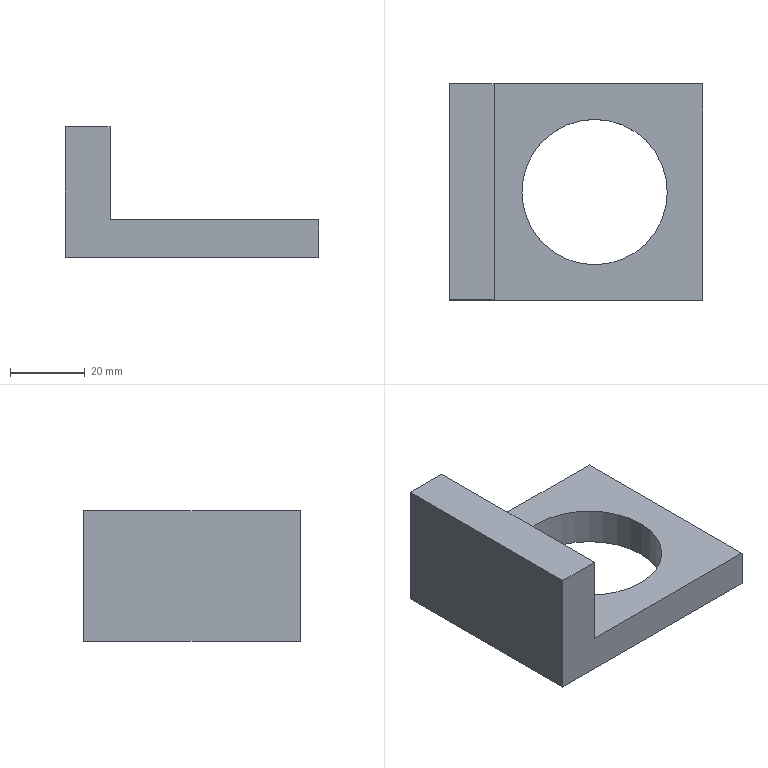Part | SolidWorks | features ICE 3, Extrusion 1 | 1 solid | 10 faces | box 68 x 58 x 35 mm | volume 44894 mm3 | plane 8 | cylinder 2 | commonest cylinder face diameters 39 x2
STEP:
#1=CARTESIAN_POINT('',(19.5,29.,0.));
#2=VERTEX_POINT('',#1);
#3=CARTESIAN_POINT('',(58.5,29.,0.));
#4=VERTEX_POINT('',#3);
#5=CARTESIAN_POINT('',(39.,29.,0.));
#6=DIRECTION('',(0.,0.,1.));
#7=DIRECTION('',(-1.,0.,0.));
#8=AXIS2_PLACEMENT_3D('',#5,#6,#7);
#9=CIRCLE('',#8,19.5);
#10=EDGE_CURVE('',#2,#4,#9,.T.);
#11=ORIENTED_EDGE('',*,*,#10,.F.);
#12=CARTESIAN_POINT('',(19.5,29.,10.));
#13=VERTEX_POINT('',#12);
#14=CARTESIAN_POINT('',(19.5,29.,-0.001));
#15=DIRECTION('',(0.,0.,1.));
#16=VECTOR('',#15,1000.);
#17=LINE('',#14,#16);
#18=EDGE_CURVE('',#2,#13,#17,.T.);
#19=ORIENTED_EDGE('',*,*,#18,.T.);
#20=CARTESIAN_POINT('',(58.5,29.,10.));
#21=VERTEX_POINT('',#20);
#22=CARTESIAN_POINT('',(39.,29.,10.));
#23=DIRECTION('',(0.,0.,1.));
#24=DIRECTION('',(1.,0.,0.));
#25=AXIS2_PLACEMENT_3D('',#22,#23,#24);
#26=CIRCLE('',#25,19.5);
#27=EDGE_CURVE('',#13,#21,#26,.T.);
#28=ORIENTED_EDGE('',*,*,#27,.T.);
#29=CARTESIAN_POINT('',(58.5,29.,-0.001));
#30=DIRECTION('',(0.,0.,1.));
#31=VECTOR('',#30,1000.);
#32=LINE('',#29,#31);
#33=EDGE_CURVE('',#4,#21,#32,.T.);
#34=ORIENTED_EDGE('',*,*,#33,.F.);
#35=EDGE_LOOP('',(#11,#19,#28,#34));
#36=FACE_OUTER_BOUND('',#35,.T.);
#37=CARTESIAN_POINT('',(39.,29.,-0.001));
#38=DIRECTION('',(0.,0.,1.));
#39=DIRECTION('',(1.,0.,0.));
#40=AXIS2_PLACEMENT_3D('',#37,#38,#39);
#41=CYLINDRICAL_SURFACE('',#40,19.5);
#42=ADVANCED_FACE('',(#36),#41,.F.);
#43=CARTESIAN_POINT('',(39.,29.,10.));
#44=DIRECTION('',(0.,0.,1.));
#45=DIRECTION('',(1.,0.,0.));
#46=AXIS2_PLACEMENT_3D('',#43,#44,#45);
#47=CIRCLE('',#46,19.5);
#48=EDGE_CURVE('',#21,#13,#47,.T.);
#49=ORIENTED_EDGE('',*,*,#48,.F.);
#50=ORIENTED_EDGE('',*,*,#27,.F.);
#51=EDGE_LOOP('',(#49,#50));
#52=FACE_BOUND('',#51,.T.);
#53=CARTESIAN_POINT('',(12.,0.,10.));
#54=VERTEX_POINT('',#53);
#55=CARTESIAN_POINT('',(12.,58.,10.));
#56=VERTEX_POINT('',#55);
#57=CARTESIAN_POINT('',(12.,58.,10.));
#58=DIRECTION('',(0.,1.,0.));
#59=VECTOR('',#58,1000.);
#60=LINE('',#57,#59);
#61=EDGE_CURVE('',#54,#56,#60,.T.);
#62=ORIENTED_EDGE('',*,*,#61,.F.);
#63=CARTESIAN_POINT('',(68.,0.,10.));
#64=VERTEX_POINT('',#63);
#65=CARTESIAN_POINT('',(68.,0.,10.));
#66=DIRECTION('',(1.,0.,0.));
#67=VECTOR('',#66,1000.);
#68=LINE('',#65,#67);
#69=EDGE_CURVE('',#54,#64,#68,.T.);
#70=ORIENTED_EDGE('',*,*,#69,.T.);
#71=CARTESIAN_POINT('',(68.,58.,10.));
#72=VERTEX_POINT('',#71);
#73=CARTESIAN_POINT('',(68.,58.,10.));
#74=DIRECTION('',(0.,1.,0.));
#75=VECTOR('',#74,1000.);
#76=LINE('',#73,#75);
#77=EDGE_CURVE('',#64,#72,#76,.T.);
#78=ORIENTED_EDGE('',*,*,#77,.T.);
#79=CARTESIAN_POINT('',(0.,58.,10.));
#80=DIRECTION('',(-1.,0.,0.));
#81=VECTOR('',#80,1000.);
#82=LINE('',#79,#81);
#83=EDGE_CURVE('',#72,#56,#82,.T.);
#84=ORIENTED_EDGE('',*,*,#83,.T.);
#85=EDGE_LOOP('',(#62,#70,#78,#84));
#86=FACE_OUTER_BOUND('',#85,.T.);
#87=CARTESIAN_POINT('',(0.,0.,10.));
#88=DIRECTION('',(0.,0.,-1.));
#89=DIRECTION('',(-1.,0.,0.));
#90=AXIS2_PLACEMENT_3D('',#87,#88,#89);
#91=PLANE('',#90);
#92=ADVANCED_FACE('',(#52,#86),#91,.F.);
#93=CARTESIAN_POINT('',(0.,0.,0.));
#94=VERTEX_POINT('',#93);
#95=CARTESIAN_POINT('',(68.,0.,0.));
#96=VERTEX_POINT('',#95);
#97=CARTESIAN_POINT('',(68.,0.,0.));
#98=DIRECTION('',(1.,0.,0.));
#99=VECTOR('',#98,1000.);
#100=LINE('',#97,#99);
#101=EDGE_CURVE('',#94,#96,#100,.T.);
#102=ORIENTED_EDGE('',*,*,#101,.T.);
#103=CARTESIAN_POINT('',(68.,0.,10.));
#104=DIRECTION('',(0.,0.,-1.));
#105=VECTOR('',#104,1000.);
#106=LINE('',#103,#105);
#107=EDGE_CURVE('',#64,#96,#106,.T.);
#108=ORIENTED_EDGE('',*,*,#107,.F.);
#109=ORIENTED_EDGE('',*,*,#69,.F.);
#110=CARTESIAN_POINT('',(12.,0.,35.));
#111=VERTEX_POINT('',#110);
#112=CARTESIAN_POINT('',(12.,0.,35.));
#113=DIRECTION('',(0.,0.,-1.));
#114=VECTOR('',#113,1000.);
#115=LINE('',#112,#114);
#116=EDGE_CURVE('',#111,#54,#115,.T.);
#117=ORIENTED_EDGE('',*,*,#116,.F.);
#118=CARTESIAN_POINT('',(0.,0.,35.));
#119=VERTEX_POINT('',#118);
#120=CARTESIAN_POINT('',(0.,0.,35.));
#121=DIRECTION('',(1.,0.,0.));
#122=VECTOR('',#121,1000.);
#123=LINE('',#120,#122);
#124=EDGE_CURVE('',#119,#111,#123,.T.);
#125=ORIENTED_EDGE('',*,*,#124,.F.);
#126=CARTESIAN_POINT('',(0.,0.,10.));
#127=DIRECTION('',(0.,0.,-1.));
#128=VECTOR('',#127,1000.);
#129=LINE('',#126,#128);
#130=EDGE_CURVE('',#119,#94,#129,.T.);
#131=ORIENTED_EDGE('',*,*,#130,.T.);
#132=EDGE_LOOP('',(#102,#108,#109,#117,#125,#131));
#133=FACE_OUTER_BOUND('',#132,.T.);
#134=CARTESIAN_POINT('',(68.,0.,10.));
#135=DIRECTION('',(0.,1.,0.));
#136=DIRECTION('',(-1.,0.,0.));
#137=AXIS2_PLACEMENT_3D('',#134,#135,#136);
#138=PLANE('',#137);
#139=ADVANCED_FACE('',(#133),#138,.F.);
#140=CARTESIAN_POINT('',(68.,58.,0.));
#141=VERTEX_POINT('',#140);
#142=CARTESIAN_POINT('',(68.,58.,0.));
#143=DIRECTION('',(0.,1.,0.));
#144=VECTOR('',#143,1000.);
#145=LINE('',#142,#144);
#146=EDGE_CURVE('',#96,#141,#145,.T.);
#147=ORIENTED_EDGE('',*,*,#146,.T.);
#148=CARTESIAN_POINT('',(68.,58.,10.));
#149=DIRECTION('',(0.,0.,-1.));
#150=VECTOR('',#149,1000.);
#151=LINE('',#148,#150);
#152=EDGE_CURVE('',#72,#141,#151,.T.);
#153=ORIENTED_EDGE('',*,*,#152,.F.);
#154=ORIENTED_EDGE('',*,*,#77,.F.);
#155=ORIENTED_EDGE('',*,*,#107,.T.);
#156=EDGE_LOOP('',(#147,#153,#154,#155));
#157=FACE_OUTER_BOUND('',#156,.T.);
#158=CARTESIAN_POINT('',(68.,58.,10.));
#159=DIRECTION('',(-1.,0.,0.));
#160=DIRECTION('',(0.,0.,1.));
#161=AXIS2_PLACEMENT_3D('',#158,#159,#160);
#162=PLANE('',#161);
#163=ADVANCED_FACE('',(#157),#162,.F.);
#164=CARTESIAN_POINT('',(0.,58.,0.));
#165=VERTEX_POINT('',#164);
#166=CARTESIAN_POINT('',(0.,58.,0.));
#167=DIRECTION('',(-1.,0.,0.));
#168=VECTOR('',#167,1000.);
#169=LINE('',#166,#168);
#170=EDGE_CURVE('',#141,#165,#169,.T.);
#171=ORIENTED_EDGE('',*,*,#170,.T.);
#172=CARTESIAN_POINT('',(0.,58.,35.));
#173=VERTEX_POINT('',#172);
#174=CARTESIAN_POINT('',(0.,58.,10.));
#175=DIRECTION('',(0.,0.,-1.));
#176=VECTOR('',#175,1000.);
#177=LINE('',#174,#176);
#178=EDGE_CURVE('',#173,#165,#177,.T.);
#179=ORIENTED_EDGE('',*,*,#178,.F.);
#180=CARTESIAN_POINT('',(12.,58.,35.));
#181=VERTEX_POINT('',#180);
#182=CARTESIAN_POINT('',(0.,58.,35.));
#183=DIRECTION('',(-1.,0.,0.));
#184=VECTOR('',#183,1000.);
#185=LINE('',#182,#184);
#186=EDGE_CURVE('',#181,#173,#185,.T.);
#187=ORIENTED_EDGE('',*,*,#186,.F.);
#188=CARTESIAN_POINT('',(12.,58.,35.));
#189=DIRECTION('',(0.,0.,-1.));
#190=VECTOR('',#189,1000.);
#191=LINE('',#188,#190);
#192=EDGE_CURVE('',#181,#56,#191,.T.);
#193=ORIENTED_EDGE('',*,*,#192,.T.);
#194=ORIENTED_EDGE('',*,*,#83,.F.);
#195=ORIENTED_EDGE('',*,*,#152,.T.);
#196=EDGE_LOOP('',(#171,#179,#187,#193,#194,#195));
#197=FACE_OUTER_BOUND('',#196,.T.);
#198=CARTESIAN_POINT('',(0.,58.,10.));
#199=DIRECTION('',(0.,-1.,0.));
#200=DIRECTION('',(1.,0.,0.));
#201=AXIS2_PLACEMENT_3D('',#198,#199,#200);
#202=PLANE('',#201);
#203=ADVANCED_FACE('',(#197),#202,.F.);
#204=CARTESIAN_POINT('',(0.,0.,0.));
#205=DIRECTION('',(0.,-1.,0.));
#206=VECTOR('',#205,1000.);
#207=LINE('',#204,#206);
#208=EDGE_CURVE('',#165,#94,#207,.T.);
#209=ORIENTED_EDGE('',*,*,#208,.T.);
#210=ORIENTED_EDGE('',*,*,#130,.F.);
#211=CARTESIAN_POINT('',(0.,58.,35.));
#212=DIRECTION('',(0.,-1.,0.));
#213=VECTOR('',#212,1000.);
#214=LINE('',#211,#213);
#215=EDGE_CURVE('',#173,#119,#214,.T.);
#216=ORIENTED_EDGE('',*,*,#215,.F.);
#217=ORIENTED_EDGE('',*,*,#178,.T.);
#218=EDGE_LOOP('',(#209,#210,#216,#217));
#219=FACE_OUTER_BOUND('',#218,.T.);
#220=CARTESIAN_POINT('',(0.,0.,10.));
#221=DIRECTION('',(1.,0.,0.));
#222=DIRECTION('',(0.,0.,-1.));
#223=AXIS2_PLACEMENT_3D('',#220,#221,#222);
#224=PLANE('',#223);
#225=ADVANCED_FACE('',(#219),#224,.F.);
#226=CARTESIAN_POINT('',(39.,29.,0.));
#227=DIRECTION('',(0.,0.,1.));
#228=DIRECTION('',(-1.,0.,0.));
#229=AXIS2_PLACEMENT_3D('',#226,#227,#228);
#230=CIRCLE('',#229,19.5);
#231=EDGE_CURVE('',#4,#2,#230,.T.);
#232=ORIENTED_EDGE('',*,*,#231,.T.);
#233=ORIENTED_EDGE('',*,*,#10,.T.);
#234=EDGE_LOOP('',(#232,#233));
#235=FACE_BOUND('',#234,.T.);
#236=ORIENTED_EDGE('',*,*,#101,.F.);
#237=ORIENTED_EDGE('',*,*,#208,.F.);
#238=ORIENTED_EDGE('',*,*,#170,.F.);
#239=ORIENTED_EDGE('',*,*,#146,.F.);
#240=EDGE_LOOP('',(#236,#237,#238,#239));
#241=FACE_OUTER_BOUND('',#240,.T.);
#242=CARTESIAN_POINT('',(0.,0.,0.));
#243=DIRECTION('',(0.,0.,-1.));
#244=DIRECTION('',(-1.,0.,0.));
#245=AXIS2_PLACEMENT_3D('',#242,#243,#244);
#246=PLANE('',#245);
#247=ADVANCED_FACE('',(#235,#241),#246,.T.);
#248=ORIENTED_EDGE('',*,*,#18,.F.);
#249=ORIENTED_EDGE('',*,*,#231,.F.);
#250=ORIENTED_EDGE('',*,*,#33,.T.);
#251=ORIENTED_EDGE('',*,*,#48,.T.);
#252=EDGE_LOOP('',(#248,#249,#250,#251));
#253=FACE_OUTER_BOUND('',#252,.T.);
#254=CARTESIAN_POINT('',(39.,29.,-0.001));
#255=DIRECTION('',(0.,0.,1.));
#256=DIRECTION('',(1.,0.,0.));
#257=AXIS2_PLACEMENT_3D('',#254,#255,#256);
#258=CYLINDRICAL_SURFACE('',#257,19.5);
#259=ADVANCED_FACE('',(#253),#258,.F.);
#260=ORIENTED_EDGE('',*,*,#61,.T.);
#261=ORIENTED_EDGE('',*,*,#192,.F.);
#262=CARTESIAN_POINT('',(12.,58.,35.));
#263=DIRECTION('',(0.,1.,0.));
#264=VECTOR('',#263,1000.);
#265=LINE('',#262,#264);
#266=EDGE_CURVE('',#111,#181,#265,.T.);
#267=ORIENTED_EDGE('',*,*,#266,.F.);
#268=ORIENTED_EDGE('',*,*,#116,.T.);
#269=EDGE_LOOP('',(#260,#261,#267,#268));
#270=FACE_OUTER_BOUND('',#269,.T.);
#271=CARTESIAN_POINT('',(12.,58.,35.));
#272=DIRECTION('',(-1.,0.,0.));
#273=DIRECTION('',(0.,-1.,0.));
#274=AXIS2_PLACEMENT_3D('',#271,#272,#273);
#275=PLANE('',#274);
#276=ADVANCED_FACE('',(#270),#275,.F.);
#277=ORIENTED_EDGE('',*,*,#215,.T.);
#278=ORIENTED_EDGE('',*,*,#124,.T.);
#279=ORIENTED_EDGE('',*,*,#266,.T.);
#280=ORIENTED_EDGE('',*,*,#186,.T.);
#281=EDGE_LOOP('',(#277,#278,#279,#280));
#282=FACE_OUTER_BOUND('',#281,.T.);
#283=CARTESIAN_POINT('',(0.,0.,35.));
#284=DIRECTION('',(0.,0.,1.));
#285=DIRECTION('',(1.,0.,0.));
#286=AXIS2_PLACEMENT_3D('',#283,#284,#285);
#287=PLANE('',#286);
#288=ADVANCED_FACE('',(#282),#287,.T.);
#289=CLOSED_SHELL('',(#42,#92,#139,#163,#203,#225,#247,#259,#276,#288));
#290=MANIFOLD_SOLID_BREP('',#289);
#291=CARTESIAN_POINT('',(0.,0.,0.));
#292=DIRECTION('',(0.,0.,1.));
#293=DIRECTION('',(1.,0.,0.));
#294=AXIS2_PLACEMENT_3D('',#291,#292,#293);
#295=(LENGTH_UNIT()NAMED_UNIT(*)SI_UNIT(.MILLI.,.METRE.));
#296=UNCERTAINTY_MEASURE_WITH_UNIT(LENGTH_MEASURE(0.00001),#295,'','');
#297=(NAMED_UNIT(*)PLANE_ANGLE_UNIT()SI_UNIT($,.RADIAN.));
#298=(NAMED_UNIT(*)SI_UNIT($,.STERADIAN.)SOLID_ANGLE_UNIT());
#299=(GEOMETRIC_REPRESENTATION_CONTEXT(3)GLOBAL_UNCERTAINTY_ASSIGNED_CONTEXT((#296))GLOBAL_UNIT_ASSIGNED_CONTEXT((#295,#297,#298))REPRESENTATION_CONTEXT('',''));
#300=ADVANCED_BREP_SHAPE_REPRESENTATION('',(#290,#294),#299);